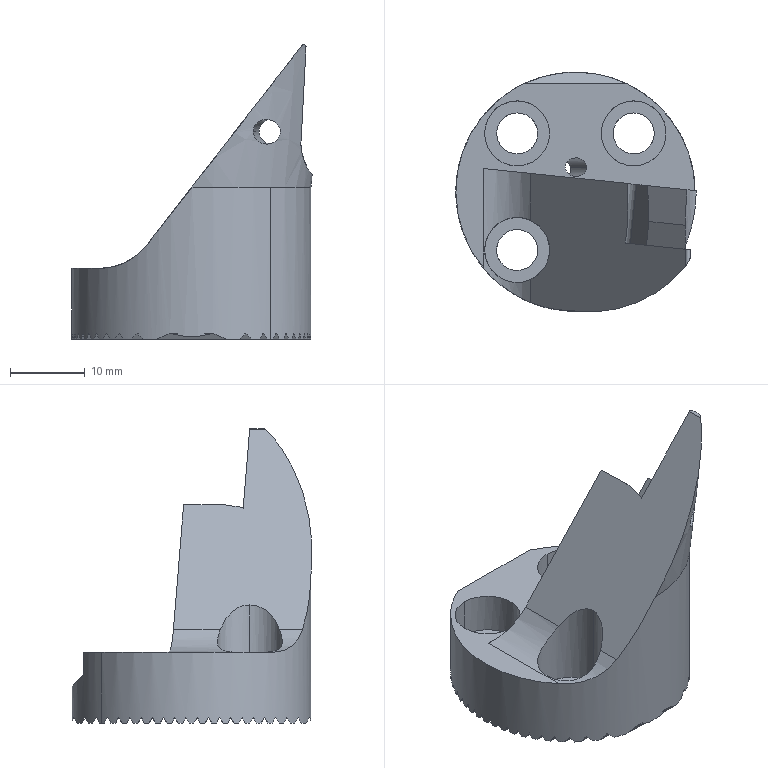Part | 1 solid | 166 faces | volume 9448 mm3 | plane 135 | cylinder 26 | cone 5 | commonest cylinder face diameters 5.5 x6 8.7 x6 2.5 x2 3.3 x2 10.5 x2 12 x2